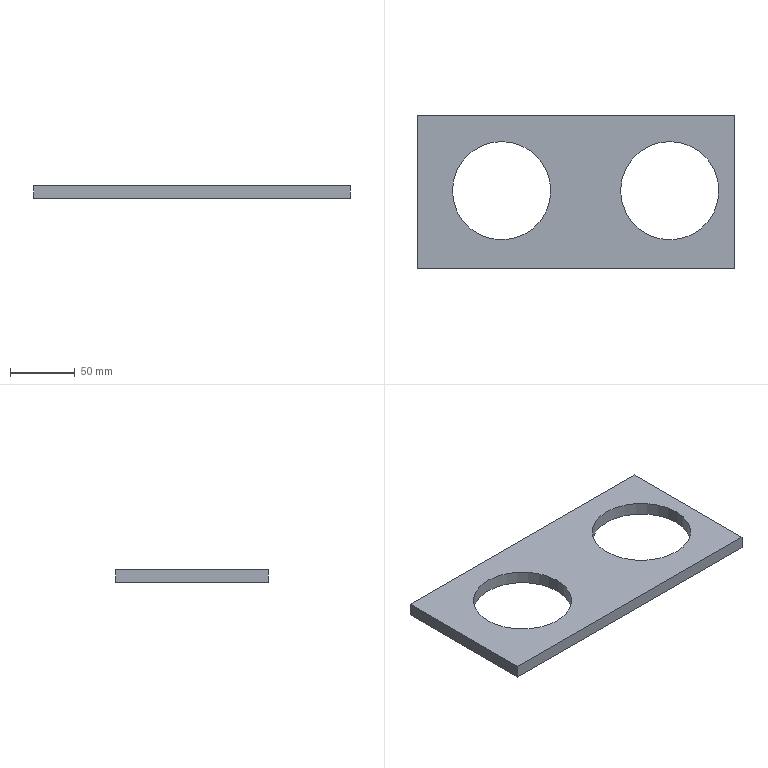Part | SolidWorks | features Extrusion 1 | 1 solid | 10 faces | box 245 x 118 x 10 mm | volume 198371 mm3 | plane 6 | cylinder 4 | commonest cylinder face diameters 76 x4
STEP:
#1=CARTESIAN_POINT('',(27.,60.,10.));
#2=VERTEX_POINT('',#1);
#3=CARTESIAN_POINT('',(103.,60.,10.));
#4=VERTEX_POINT('',#3);
#5=CARTESIAN_POINT('',(65.,60.,10.));
#6=DIRECTION('',(0.,0.,1.));
#7=DIRECTION('',(1.,0.,0.));
#8=AXIS2_PLACEMENT_3D('',#5,#6,#7);
#9=CIRCLE('',#8,38.);
#10=EDGE_CURVE('',#2,#4,#9,.T.);
#11=ORIENTED_EDGE('',*,*,#10,.T.);
#12=CARTESIAN_POINT('',(103.,60.,0.));
#13=VERTEX_POINT('',#12);
#14=CARTESIAN_POINT('',(103.,60.,10.));
#15=DIRECTION('',(0.,0.,-1.));
#16=VECTOR('',#15,1000.);
#17=LINE('',#14,#16);
#18=EDGE_CURVE('',#4,#13,#17,.T.);
#19=ORIENTED_EDGE('',*,*,#18,.T.);
#20=CARTESIAN_POINT('',(27.,60.,0.));
#21=VERTEX_POINT('',#20);
#22=CARTESIAN_POINT('',(65.,60.,0.));
#23=DIRECTION('',(0.,0.,1.));
#24=DIRECTION('',(1.,0.,0.));
#25=AXIS2_PLACEMENT_3D('',#22,#23,#24);
#26=CIRCLE('',#25,38.);
#27=EDGE_CURVE('',#21,#13,#26,.T.);
#28=ORIENTED_EDGE('',*,*,#27,.F.);
#29=CARTESIAN_POINT('',(27.,60.,10.));
#30=DIRECTION('',(0.,0.,-1.));
#31=VECTOR('',#30,1000.);
#32=LINE('',#29,#31);
#33=EDGE_CURVE('',#2,#21,#32,.T.);
#34=ORIENTED_EDGE('',*,*,#33,.F.);
#35=EDGE_LOOP('',(#11,#19,#28,#34));
#36=FACE_OUTER_BOUND('',#35,.T.);
#37=CARTESIAN_POINT('',(65.,60.,10.));
#38=DIRECTION('',(0.,0.,-1.));
#39=DIRECTION('',(-1.,0.,0.));
#40=AXIS2_PLACEMENT_3D('',#37,#38,#39);
#41=CYLINDRICAL_SURFACE('',#40,38.);
#42=ADVANCED_FACE('',(#36),#41,.F.);
#43=CARTESIAN_POINT('',(157.,60.,10.));
#44=VERTEX_POINT('',#43);
#45=CARTESIAN_POINT('',(233.,60.,10.));
#46=VERTEX_POINT('',#45);
#47=CARTESIAN_POINT('',(195.,60.,10.));
#48=DIRECTION('',(0.,0.,1.));
#49=DIRECTION('',(1.,0.,0.));
#50=AXIS2_PLACEMENT_3D('',#47,#48,#49);
#51=CIRCLE('',#50,38.);
#52=EDGE_CURVE('',#44,#46,#51,.T.);
#53=ORIENTED_EDGE('',*,*,#52,.T.);
#54=CARTESIAN_POINT('',(233.,60.,0.));
#55=VERTEX_POINT('',#54);
#56=CARTESIAN_POINT('',(233.,60.,10.));
#57=DIRECTION('',(0.,0.,-1.));
#58=VECTOR('',#57,1000.);
#59=LINE('',#56,#58);
#60=EDGE_CURVE('',#46,#55,#59,.T.);
#61=ORIENTED_EDGE('',*,*,#60,.T.);
#62=CARTESIAN_POINT('',(157.,60.,0.));
#63=VERTEX_POINT('',#62);
#64=CARTESIAN_POINT('',(195.,60.,0.));
#65=DIRECTION('',(0.,0.,1.));
#66=DIRECTION('',(1.,0.,0.));
#67=AXIS2_PLACEMENT_3D('',#64,#65,#66);
#68=CIRCLE('',#67,38.);
#69=EDGE_CURVE('',#63,#55,#68,.T.);
#70=ORIENTED_EDGE('',*,*,#69,.F.);
#71=CARTESIAN_POINT('',(157.,60.,10.));
#72=DIRECTION('',(0.,0.,-1.));
#73=VECTOR('',#72,1000.);
#74=LINE('',#71,#73);
#75=EDGE_CURVE('',#44,#63,#74,.T.);
#76=ORIENTED_EDGE('',*,*,#75,.F.);
#77=EDGE_LOOP('',(#53,#61,#70,#76));
#78=FACE_OUTER_BOUND('',#77,.T.);
#79=CARTESIAN_POINT('',(195.,60.,10.));
#80=DIRECTION('',(0.,0.,-1.));
#81=DIRECTION('',(-1.,0.,0.));
#82=AXIS2_PLACEMENT_3D('',#79,#80,#81);
#83=CYLINDRICAL_SURFACE('',#82,38.);
#84=ADVANCED_FACE('',(#78),#83,.F.);
#85=ORIENTED_EDGE('',*,*,#52,.F.);
#86=CARTESIAN_POINT('',(195.,60.,10.));
#87=DIRECTION('',(0.,0.,1.));
#88=DIRECTION('',(1.,0.,0.));
#89=AXIS2_PLACEMENT_3D('',#86,#87,#88);
#90=CIRCLE('',#89,38.);
#91=EDGE_CURVE('',#46,#44,#90,.T.);
#92=ORIENTED_EDGE('',*,*,#91,.F.);
#93=EDGE_LOOP('',(#85,#92));
#94=FACE_BOUND('',#93,.T.);
#95=CARTESIAN_POINT('',(0.,118.,10.));
#96=VERTEX_POINT('',#95);
#97=CARTESIAN_POINT('',(0.,0.,10.));
#98=VERTEX_POINT('',#97);
#99=CARTESIAN_POINT('',(0.,0.,10.));
#100=DIRECTION('',(0.,-1.,0.));
#101=VECTOR('',#100,1000.);
#102=LINE('',#99,#101);
#103=EDGE_CURVE('',#96,#98,#102,.T.);
#104=ORIENTED_EDGE('',*,*,#103,.T.);
#105=CARTESIAN_POINT('',(245.,0.,10.));
#106=VERTEX_POINT('',#105);
#107=CARTESIAN_POINT('',(0.,0.,10.));
#108=DIRECTION('',(1.,0.,0.));
#109=VECTOR('',#108,1000.);
#110=LINE('',#107,#109);
#111=EDGE_CURVE('',#98,#106,#110,.T.);
#112=ORIENTED_EDGE('',*,*,#111,.T.);
#113=CARTESIAN_POINT('',(245.,118.,10.));
#114=VERTEX_POINT('',#113);
#115=CARTESIAN_POINT('',(245.,0.,10.));
#116=DIRECTION('',(0.,1.,0.));
#117=VECTOR('',#116,1000.);
#118=LINE('',#115,#117);
#119=EDGE_CURVE('',#106,#114,#118,.T.);
#120=ORIENTED_EDGE('',*,*,#119,.T.);
#121=CARTESIAN_POINT('',(0.,118.,10.));
#122=DIRECTION('',(-1.,0.,0.));
#123=VECTOR('',#122,1000.);
#124=LINE('',#121,#123);
#125=EDGE_CURVE('',#114,#96,#124,.T.);
#126=ORIENTED_EDGE('',*,*,#125,.T.);
#127=EDGE_LOOP('',(#104,#112,#120,#126));
#128=FACE_OUTER_BOUND('',#127,.T.);
#129=ORIENTED_EDGE('',*,*,#10,.F.);
#130=CARTESIAN_POINT('',(65.,60.,10.));
#131=DIRECTION('',(0.,0.,1.));
#132=DIRECTION('',(1.,0.,0.));
#133=AXIS2_PLACEMENT_3D('',#130,#131,#132);
#134=CIRCLE('',#133,38.);
#135=EDGE_CURVE('',#4,#2,#134,.T.);
#136=ORIENTED_EDGE('',*,*,#135,.F.);
#137=EDGE_LOOP('',(#129,#136));
#138=FACE_BOUND('',#137,.T.);
#139=CARTESIAN_POINT('',(0.,118.,10.));
#140=DIRECTION('',(0.,0.,-1.));
#141=DIRECTION('',(-1.,0.,0.));
#142=AXIS2_PLACEMENT_3D('',#139,#140,#141);
#143=PLANE('',#142);
#144=ADVANCED_FACE('',(#94,#128,#138),#143,.F.);
#145=ORIENTED_EDGE('',*,*,#69,.T.);
#146=CARTESIAN_POINT('',(195.,60.,0.));
#147=DIRECTION('',(0.,0.,1.));
#148=DIRECTION('',(1.,0.,0.));
#149=AXIS2_PLACEMENT_3D('',#146,#147,#148);
#150=CIRCLE('',#149,38.);
#151=EDGE_CURVE('',#55,#63,#150,.T.);
#152=ORIENTED_EDGE('',*,*,#151,.T.);
#153=EDGE_LOOP('',(#145,#152));
#154=FACE_BOUND('',#153,.T.);
#155=CARTESIAN_POINT('',(0.,118.,0.));
#156=VERTEX_POINT('',#155);
#157=CARTESIAN_POINT('',(0.,0.,0.));
#158=VERTEX_POINT('',#157);
#159=CARTESIAN_POINT('',(0.,0.,0.));
#160=DIRECTION('',(0.,-1.,0.));
#161=VECTOR('',#160,1000.);
#162=LINE('',#159,#161);
#163=EDGE_CURVE('',#156,#158,#162,.T.);
#164=ORIENTED_EDGE('',*,*,#163,.F.);
#165=CARTESIAN_POINT('',(245.,118.,0.));
#166=VERTEX_POINT('',#165);
#167=CARTESIAN_POINT('',(0.,118.,0.));
#168=DIRECTION('',(-1.,0.,0.));
#169=VECTOR('',#168,1000.);
#170=LINE('',#167,#169);
#171=EDGE_CURVE('',#166,#156,#170,.T.);
#172=ORIENTED_EDGE('',*,*,#171,.F.);
#173=CARTESIAN_POINT('',(245.,0.,0.));
#174=VERTEX_POINT('',#173);
#175=CARTESIAN_POINT('',(245.,0.,0.));
#176=DIRECTION('',(0.,1.,0.));
#177=VECTOR('',#176,1000.);
#178=LINE('',#175,#177);
#179=EDGE_CURVE('',#174,#166,#178,.T.);
#180=ORIENTED_EDGE('',*,*,#179,.F.);
#181=CARTESIAN_POINT('',(0.,0.,0.));
#182=DIRECTION('',(1.,0.,0.));
#183=VECTOR('',#182,1000.);
#184=LINE('',#181,#183);
#185=EDGE_CURVE('',#158,#174,#184,.T.);
#186=ORIENTED_EDGE('',*,*,#185,.F.);
#187=EDGE_LOOP('',(#164,#172,#180,#186));
#188=FACE_OUTER_BOUND('',#187,.T.);
#189=ORIENTED_EDGE('',*,*,#27,.T.);
#190=CARTESIAN_POINT('',(65.,60.,0.));
#191=DIRECTION('',(0.,0.,1.));
#192=DIRECTION('',(1.,0.,0.));
#193=AXIS2_PLACEMENT_3D('',#190,#191,#192);
#194=CIRCLE('',#193,38.);
#195=EDGE_CURVE('',#13,#21,#194,.T.);
#196=ORIENTED_EDGE('',*,*,#195,.T.);
#197=EDGE_LOOP('',(#189,#196));
#198=FACE_BOUND('',#197,.T.);
#199=CARTESIAN_POINT('',(0.,118.,0.));
#200=DIRECTION('',(0.,0.,-1.));
#201=DIRECTION('',(-1.,0.,0.));
#202=AXIS2_PLACEMENT_3D('',#199,#200,#201);
#203=PLANE('',#202);
#204=ADVANCED_FACE('',(#154,#188,#198),#203,.T.);
#205=ORIENTED_EDGE('',*,*,#163,.T.);
#206=CARTESIAN_POINT('',(0.,0.,10.));
#207=DIRECTION('',(0.,0.,-1.));
#208=VECTOR('',#207,1000.);
#209=LINE('',#206,#208);
#210=EDGE_CURVE('',#98,#158,#209,.T.);
#211=ORIENTED_EDGE('',*,*,#210,.F.);
#212=ORIENTED_EDGE('',*,*,#103,.F.);
#213=CARTESIAN_POINT('',(0.,118.,10.));
#214=DIRECTION('',(0.,0.,-1.));
#215=VECTOR('',#214,1000.);
#216=LINE('',#213,#215);
#217=EDGE_CURVE('',#96,#156,#216,.T.);
#218=ORIENTED_EDGE('',*,*,#217,.T.);
#219=EDGE_LOOP('',(#205,#211,#212,#218));
#220=FACE_OUTER_BOUND('',#219,.T.);
#221=CARTESIAN_POINT('',(0.,0.,10.));
#222=DIRECTION('',(1.,0.,0.));
#223=DIRECTION('',(0.,0.,-1.));
#224=AXIS2_PLACEMENT_3D('',#221,#222,#223);
#225=PLANE('',#224);
#226=ADVANCED_FACE('',(#220),#225,.F.);
#227=ORIENTED_EDGE('',*,*,#185,.T.);
#228=CARTESIAN_POINT('',(245.,0.,10.));
#229=DIRECTION('',(0.,0.,-1.));
#230=VECTOR('',#229,1000.);
#231=LINE('',#228,#230);
#232=EDGE_CURVE('',#106,#174,#231,.T.);
#233=ORIENTED_EDGE('',*,*,#232,.F.);
#234=ORIENTED_EDGE('',*,*,#111,.F.);
#235=ORIENTED_EDGE('',*,*,#210,.T.);
#236=EDGE_LOOP('',(#227,#233,#234,#235));
#237=FACE_OUTER_BOUND('',#236,.T.);
#238=CARTESIAN_POINT('',(0.,0.,10.));
#239=DIRECTION('',(0.,1.,0.));
#240=DIRECTION('',(0.,0.,1.));
#241=AXIS2_PLACEMENT_3D('',#238,#239,#240);
#242=PLANE('',#241);
#243=ADVANCED_FACE('',(#237),#242,.F.);
#244=ORIENTED_EDGE('',*,*,#179,.T.);
#245=CARTESIAN_POINT('',(245.,118.,10.));
#246=DIRECTION('',(0.,0.,-1.));
#247=VECTOR('',#246,1000.);
#248=LINE('',#245,#247);
#249=EDGE_CURVE('',#114,#166,#248,.T.);
#250=ORIENTED_EDGE('',*,*,#249,.F.);
#251=ORIENTED_EDGE('',*,*,#119,.F.);
#252=ORIENTED_EDGE('',*,*,#232,.T.);
#253=EDGE_LOOP('',(#244,#250,#251,#252));
#254=FACE_OUTER_BOUND('',#253,.T.);
#255=CARTESIAN_POINT('',(245.,0.,10.));
#256=DIRECTION('',(-1.,0.,0.));
#257=DIRECTION('',(0.,0.,1.));
#258=AXIS2_PLACEMENT_3D('',#255,#256,#257);
#259=PLANE('',#258);
#260=ADVANCED_FACE('',(#254),#259,.F.);
#261=ORIENTED_EDGE('',*,*,#171,.T.);
#262=ORIENTED_EDGE('',*,*,#217,.F.);
#263=ORIENTED_EDGE('',*,*,#125,.F.);
#264=ORIENTED_EDGE('',*,*,#249,.T.);
#265=EDGE_LOOP('',(#261,#262,#263,#264));
#266=FACE_OUTER_BOUND('',#265,.T.);
#267=CARTESIAN_POINT('',(0.,118.,10.));
#268=DIRECTION('',(0.,-1.,0.));
#269=DIRECTION('',(0.,0.,-1.));
#270=AXIS2_PLACEMENT_3D('',#267,#268,#269);
#271=PLANE('',#270);
#272=ADVANCED_FACE('',(#266),#271,.F.);
#273=ORIENTED_EDGE('',*,*,#60,.F.);
#274=ORIENTED_EDGE('',*,*,#91,.T.);
#275=ORIENTED_EDGE('',*,*,#75,.T.);
#276=ORIENTED_EDGE('',*,*,#151,.F.);
#277=EDGE_LOOP('',(#273,#274,#275,#276));
#278=FACE_OUTER_BOUND('',#277,.T.);
#279=CARTESIAN_POINT('',(195.,60.,10.));
#280=DIRECTION('',(0.,0.,-1.));
#281=DIRECTION('',(-1.,0.,0.));
#282=AXIS2_PLACEMENT_3D('',#279,#280,#281);
#283=CYLINDRICAL_SURFACE('',#282,38.);
#284=ADVANCED_FACE('',(#278),#283,.F.);
#285=ORIENTED_EDGE('',*,*,#18,.F.);
#286=ORIENTED_EDGE('',*,*,#135,.T.);
#287=ORIENTED_EDGE('',*,*,#33,.T.);
#288=ORIENTED_EDGE('',*,*,#195,.F.);
#289=EDGE_LOOP('',(#285,#286,#287,#288));
#290=FACE_OUTER_BOUND('',#289,.T.);
#291=CARTESIAN_POINT('',(65.,60.,10.));
#292=DIRECTION('',(0.,0.,-1.));
#293=DIRECTION('',(-1.,0.,0.));
#294=AXIS2_PLACEMENT_3D('',#291,#292,#293);
#295=CYLINDRICAL_SURFACE('',#294,38.);
#296=ADVANCED_FACE('',(#290),#295,.F.);
#297=CLOSED_SHELL('',(#42,#84,#144,#204,#226,#243,#260,#272,#284,#296));
#298=MANIFOLD_SOLID_BREP('',#297);
#299=CARTESIAN_POINT('',(0.,0.,0.));
#300=DIRECTION('',(0.,0.,1.));
#301=DIRECTION('',(1.,0.,0.));
#302=AXIS2_PLACEMENT_3D('',#299,#300,#301);
#303=(LENGTH_UNIT()NAMED_UNIT(*)SI_UNIT(.MILLI.,.METRE.));
#304=UNCERTAINTY_MEASURE_WITH_UNIT(LENGTH_MEASURE(0.00001),#303,'','');
#305=(NAMED_UNIT(*)PLANE_ANGLE_UNIT()SI_UNIT($,.RADIAN.));
#306=(NAMED_UNIT(*)SI_UNIT($,.STERADIAN.)SOLID_ANGLE_UNIT());
#307=(GEOMETRIC_REPRESENTATION_CONTEXT(3)GLOBAL_UNCERTAINTY_ASSIGNED_CONTEXT((#304))GLOBAL_UNIT_ASSIGNED_CONTEXT((#303,#305,#306))REPRESENTATION_CONTEXT('',''));
#308=ADVANCED_BREP_SHAPE_REPRESENTATION('',(#298,#302),#307);